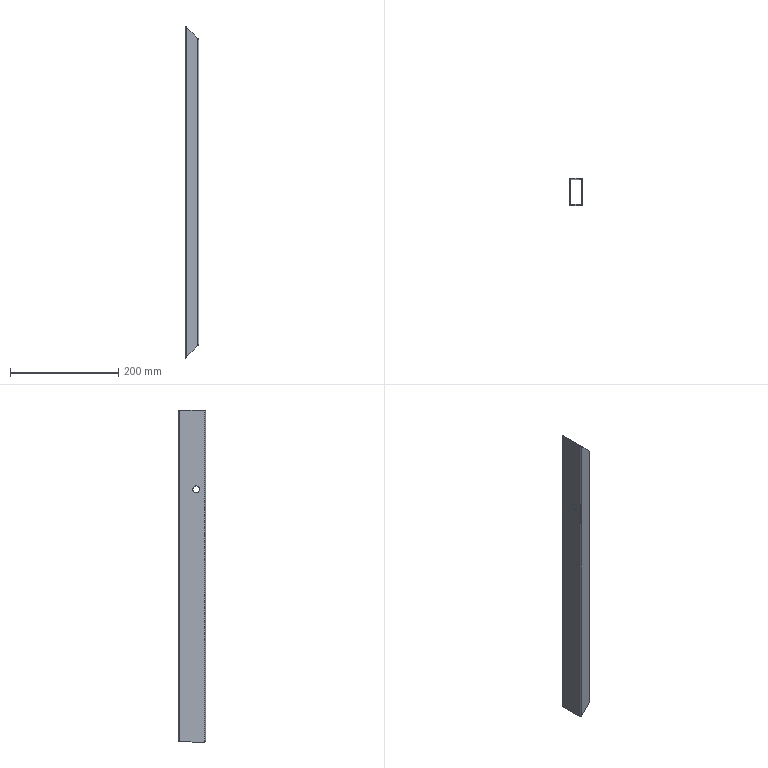Part | STEP file | 6150519 | 1 solid | 20 faces | box 25 x 50 x 613 mm | volume 123960 mm3 | cylinder 10 | plane 10 | commonest cylinder face diameters 2 x4 5 x4 13 x2
STEP:
#1=CARTESIAN_POINT('',(-10.,-25.,610.5));
#2=VERTEX_POINT('',#1);
#3=CARTESIAN_POINT('',(-10.,-25.,2.5));
#4=VERTEX_POINT('',#3);
#5=CARTESIAN_POINT('',(-10.,-25.,613.));
#6=DIRECTION('',(0.,0.,-1.));
#7=VECTOR('',#6,1000.);
#8=LINE('',#5,#7);
#9=EDGE_CURVE('',#2,#4,#8,.T.);
#10=ORIENTED_EDGE('',*,*,#9,.F.);
#11=CARTESIAN_POINT('',(-12.5,-22.5,613.));
#12=VERTEX_POINT('',#11);
#13=CARTESIAN_POINT('',(-10.,-25.,610.5));
#14=CARTESIAN_POINT('',(-11.464,-25.,611.964));
#15=CARTESIAN_POINT('',(-12.5,-23.964,613.));
#16=CARTESIAN_POINT('',(-12.5,-22.5,613.));
#17=(BOUNDED_CURVE()B_SPLINE_CURVE(3,(#13,#14,#15,#16),.UNSPECIFIED.,.F.,.F.)B_SPLINE_CURVE_WITH_KNOTS((4,4),(1.571,3.142),.UNSPECIFIED.)CURVE()GEOMETRIC_REPRESENTATION_ITEM()RATIONAL_B_SPLINE_CURVE((1.,0.8047,0.8047,1.))REPRESENTATION_ITEM(''));
#18=EDGE_CURVE('',#2,#12,#17,.T.);
#19=ORIENTED_EDGE('',*,*,#18,.T.);
#20=CARTESIAN_POINT('',(-12.5,-22.5,0.));
#21=VERTEX_POINT('',#20);
#22=CARTESIAN_POINT('',(-12.5,-22.5,613.));
#23=DIRECTION('',(0.,0.,-1.));
#24=VECTOR('',#23,1000.);
#25=LINE('',#22,#24);
#26=EDGE_CURVE('',#12,#21,#25,.T.);
#27=ORIENTED_EDGE('',*,*,#26,.T.);
#28=CARTESIAN_POINT('',(-10.,-25.,2.5));
#29=CARTESIAN_POINT('',(-11.464,-25.,1.036));
#30=CARTESIAN_POINT('',(-12.5,-23.964,0.));
#31=CARTESIAN_POINT('',(-12.5,-22.5,0.));
#32=(BOUNDED_CURVE()B_SPLINE_CURVE(3,(#28,#29,#30,#31),.UNSPECIFIED.,.F.,.F.)B_SPLINE_CURVE_WITH_KNOTS((4,4),(4.712,6.283),.UNSPECIFIED.)CURVE()GEOMETRIC_REPRESENTATION_ITEM()RATIONAL_B_SPLINE_CURVE((1.,0.8047,0.8047,1.))REPRESENTATION_ITEM(''));
#33=EDGE_CURVE('',#4,#21,#32,.T.);
#34=ORIENTED_EDGE('',*,*,#33,.F.);
#35=EDGE_LOOP('',(#10,#19,#27,#34));
#36=FACE_OUTER_BOUND('',#35,.T.);
#37=CARTESIAN_POINT('',(-10.,-22.5,613.));
#38=DIRECTION('',(0.,0.,-1.));
#39=DIRECTION('',(-1.,0.,0.));
#40=AXIS2_PLACEMENT_3D('',#37,#38,#39);
#41=CYLINDRICAL_SURFACE('',#40,2.5);
#42=ADVANCED_FACE('',(#36),#41,.T.);
#43=CARTESIAN_POINT('',(10.,-25.,590.5));
#44=VERTEX_POINT('',#43);
#45=CARTESIAN_POINT('',(10.,-25.,22.5));
#46=VERTEX_POINT('',#45);
#47=CARTESIAN_POINT('',(10.,-25.,613.));
#48=DIRECTION('',(0.,0.,-1.));
#49=VECTOR('',#48,1000.);
#50=LINE('',#47,#49);
#51=EDGE_CURVE('',#44,#46,#50,.T.);
#52=ORIENTED_EDGE('',*,*,#51,.F.);
#53=CARTESIAN_POINT('',(-11.25,-25.,611.75));
#54=DIRECTION('',(-0.7071,0.,0.7071));
#55=VECTOR('',#54,1000.);
#56=LINE('',#53,#55);
#57=EDGE_CURVE('',#44,#2,#56,.T.);
#58=ORIENTED_EDGE('',*,*,#57,.T.);
#59=ORIENTED_EDGE('',*,*,#9,.T.);
#60=CARTESIAN_POINT('',(295.25,-25.,307.75));
#61=DIRECTION('',(-0.7071,0.,-0.7071));
#62=VECTOR('',#61,1000.);
#63=LINE('',#60,#62);
#64=EDGE_CURVE('',#46,#4,#63,.T.);
#65=ORIENTED_EDGE('',*,*,#64,.F.);
#66=EDGE_LOOP('',(#52,#58,#59,#65));
#67=FACE_OUTER_BOUND('',#66,.T.);
#68=CARTESIAN_POINT('',(-10.,-25.,613.));
#69=DIRECTION('',(0.,1.,0.));
#70=DIRECTION('',(0.,0.,1.));
#71=AXIS2_PLACEMENT_3D('',#68,#69,#70);
#72=PLANE('',#71);
#73=ADVANCED_FACE('',(#67),#72,.F.);
#74=CARTESIAN_POINT('',(12.5,-22.5,588.));
#75=VERTEX_POINT('',#74);
#76=CARTESIAN_POINT('',(12.5,-22.5,25.));
#77=VERTEX_POINT('',#76);
#78=CARTESIAN_POINT('',(12.5,-22.5,613.));
#79=DIRECTION('',(0.,0.,-1.));
#80=VECTOR('',#79,1000.);
#81=LINE('',#78,#80);
#82=EDGE_CURVE('',#75,#77,#81,.T.);
#83=ORIENTED_EDGE('',*,*,#82,.F.);
#84=CARTESIAN_POINT('',(12.5,-22.5,588.));
#85=CARTESIAN_POINT('',(12.5,-23.964,588.));
#86=CARTESIAN_POINT('',(11.464,-25.,589.036));
#87=CARTESIAN_POINT('',(10.,-25.,590.5));
#88=(BOUNDED_CURVE()B_SPLINE_CURVE(3,(#84,#85,#86,#87),.UNSPECIFIED.,.F.,.T.)B_SPLINE_CURVE_WITH_KNOTS((4,4),(0.,1.571),.UNSPECIFIED.)CURVE()GEOMETRIC_REPRESENTATION_ITEM()RATIONAL_B_SPLINE_CURVE((1.,0.8047,0.8047,1.))REPRESENTATION_ITEM(''));
#89=EDGE_CURVE('',#75,#44,#88,.T.);
#90=ORIENTED_EDGE('',*,*,#89,.T.);
#91=ORIENTED_EDGE('',*,*,#51,.T.);
#92=CARTESIAN_POINT('',(12.5,-22.5,25.));
#93=CARTESIAN_POINT('',(12.5,-23.964,25.));
#94=CARTESIAN_POINT('',(11.464,-25.,23.964));
#95=CARTESIAN_POINT('',(10.,-25.,22.5));
#96=(BOUNDED_CURVE()B_SPLINE_CURVE(3,(#92,#93,#94,#95),.UNSPECIFIED.,.F.,.F.)B_SPLINE_CURVE_WITH_KNOTS((4,4),(3.142,4.712),.UNSPECIFIED.)CURVE()GEOMETRIC_REPRESENTATION_ITEM()RATIONAL_B_SPLINE_CURVE((1.,0.8047,0.8047,1.))REPRESENTATION_ITEM(''));
#97=EDGE_CURVE('',#77,#46,#96,.T.);
#98=ORIENTED_EDGE('',*,*,#97,.F.);
#99=EDGE_LOOP('',(#83,#90,#91,#98));
#100=FACE_OUTER_BOUND('',#99,.T.);
#101=CARTESIAN_POINT('',(10.,-22.5,613.));
#102=DIRECTION('',(0.,0.,-1.));
#103=DIRECTION('',(-1.,0.,0.));
#104=AXIS2_PLACEMENT_3D('',#101,#102,#103);
#105=CYLINDRICAL_SURFACE('',#104,2.5);
#106=ADVANCED_FACE('',(#100),#105,.T.);
#107=CARTESIAN_POINT('',(12.5,-14.5,466.5));
#108=VERTEX_POINT('',#107);
#109=CARTESIAN_POINT('',(12.5,-8.,466.5));
#110=DIRECTION('',(-1.,0.,0.));
#111=DIRECTION('',(0.,-1.,0.));
#112=AXIS2_PLACEMENT_3D('',#109,#110,#111);
#113=CIRCLE('',#112,6.5);
#114=EDGE_CURVE('',#108,#108,#113,.T.);
#115=ORIENTED_EDGE('',*,*,#114,.T.);
#116=EDGE_LOOP('',(#115));
#117=FACE_BOUND('',#116,.T.);
#118=CARTESIAN_POINT('',(12.5,22.5,588.));
#119=VERTEX_POINT('',#118);
#120=CARTESIAN_POINT('',(12.5,22.5,25.));
#121=VERTEX_POINT('',#120);
#122=CARTESIAN_POINT('',(12.5,22.5,613.));
#123=DIRECTION('',(0.,0.,-1.));
#124=VECTOR('',#123,1000.);
#125=LINE('',#122,#124);
#126=EDGE_CURVE('',#119,#121,#125,.T.);
#127=ORIENTED_EDGE('',*,*,#126,.F.);
#128=CARTESIAN_POINT('',(12.5,22.5,588.));
#129=DIRECTION('',(0.,-1.,0.));
#130=VECTOR('',#129,1000.);
#131=LINE('',#128,#130);
#132=EDGE_CURVE('',#119,#75,#131,.T.);
#133=ORIENTED_EDGE('',*,*,#132,.T.);
#134=ORIENTED_EDGE('',*,*,#82,.T.);
#135=CARTESIAN_POINT('',(12.5,22.5,25.));
#136=DIRECTION('',(0.,-1.,0.));
#137=VECTOR('',#136,1000.);
#138=LINE('',#135,#137);
#139=EDGE_CURVE('',#121,#77,#138,.T.);
#140=ORIENTED_EDGE('',*,*,#139,.F.);
#141=EDGE_LOOP('',(#127,#133,#134,#140));
#142=FACE_OUTER_BOUND('',#141,.T.);
#143=CARTESIAN_POINT('',(12.5,22.5,613.));
#144=DIRECTION('',(-1.,0.,0.));
#145=DIRECTION('',(0.,-1.,0.));
#146=AXIS2_PLACEMENT_3D('',#143,#144,#145);
#147=PLANE('',#146);
#148=ADVANCED_FACE('',(#117,#142),#147,.F.);
#149=CARTESIAN_POINT('',(10.,25.,590.5));
#150=VERTEX_POINT('',#149);
#151=CARTESIAN_POINT('',(10.,25.,22.5));
#152=VERTEX_POINT('',#151);
#153=CARTESIAN_POINT('',(10.,25.,613.));
#154=DIRECTION('',(0.,0.,-1.));
#155=VECTOR('',#154,1000.);
#156=LINE('',#153,#155);
#157=EDGE_CURVE('',#150,#152,#156,.T.);
#158=ORIENTED_EDGE('',*,*,#157,.F.);
#159=CARTESIAN_POINT('',(10.,25.,590.5));
#160=CARTESIAN_POINT('',(11.464,25.,589.036));
#161=CARTESIAN_POINT('',(12.5,23.964,588.));
#162=CARTESIAN_POINT('',(12.5,22.5,588.));
#163=(BOUNDED_CURVE()B_SPLINE_CURVE(3,(#159,#160,#161,#162),.UNSPECIFIED.,.F.,.F.)B_SPLINE_CURVE_WITH_KNOTS((4,4),(4.712,6.283),.UNSPECIFIED.)CURVE()GEOMETRIC_REPRESENTATION_ITEM()RATIONAL_B_SPLINE_CURVE((1.,0.8047,0.8047,1.))REPRESENTATION_ITEM(''));
#164=EDGE_CURVE('',#150,#119,#163,.T.);
#165=ORIENTED_EDGE('',*,*,#164,.T.);
#166=ORIENTED_EDGE('',*,*,#126,.T.);
#167=CARTESIAN_POINT('',(10.,25.,22.5));
#168=CARTESIAN_POINT('',(11.464,25.,23.964));
#169=CARTESIAN_POINT('',(12.5,23.964,25.));
#170=CARTESIAN_POINT('',(12.5,22.5,25.));
#171=(BOUNDED_CURVE()B_SPLINE_CURVE(3,(#167,#168,#169,#170),.UNSPECIFIED.,.F.,.F.)B_SPLINE_CURVE_WITH_KNOTS((4,4),(1.571,3.142),.UNSPECIFIED.)CURVE()GEOMETRIC_REPRESENTATION_ITEM()RATIONAL_B_SPLINE_CURVE((1.,0.8047,0.8047,1.))REPRESENTATION_ITEM(''));
#172=EDGE_CURVE('',#152,#121,#171,.T.);
#173=ORIENTED_EDGE('',*,*,#172,.F.);
#174=EDGE_LOOP('',(#158,#165,#166,#173));
#175=FACE_OUTER_BOUND('',#174,.T.);
#176=CARTESIAN_POINT('',(10.,22.5,613.));
#177=DIRECTION('',(0.,0.,-1.));
#178=DIRECTION('',(-1.,0.,0.));
#179=AXIS2_PLACEMENT_3D('',#176,#177,#178);
#180=CYLINDRICAL_SURFACE('',#179,2.5);
#181=ADVANCED_FACE('',(#175),#180,.T.);
#182=CARTESIAN_POINT('',(-10.,25.,610.5));
#183=VERTEX_POINT('',#182);
#184=CARTESIAN_POINT('',(-10.,25.,2.5));
#185=VERTEX_POINT('',#184);
#186=CARTESIAN_POINT('',(-10.,25.,613.));
#187=DIRECTION('',(0.,0.,-1.));
#188=VECTOR('',#187,1000.);
#189=LINE('',#186,#188);
#190=EDGE_CURVE('',#183,#185,#189,.T.);
#191=ORIENTED_EDGE('',*,*,#190,.F.);
#192=CARTESIAN_POINT('',(-11.25,25.,611.75));
#193=DIRECTION('',(0.7071,0.,-0.7071));
#194=VECTOR('',#193,1000.);
#195=LINE('',#192,#194);
#196=EDGE_CURVE('',#183,#150,#195,.T.);
#197=ORIENTED_EDGE('',*,*,#196,.T.);
#198=ORIENTED_EDGE('',*,*,#157,.T.);
#199=CARTESIAN_POINT('',(295.25,25.,307.75));
#200=DIRECTION('',(0.7071,0.,0.7071));
#201=VECTOR('',#200,1000.);
#202=LINE('',#199,#201);
#203=EDGE_CURVE('',#185,#152,#202,.T.);
#204=ORIENTED_EDGE('',*,*,#203,.F.);
#205=EDGE_LOOP('',(#191,#197,#198,#204));
#206=FACE_OUTER_BOUND('',#205,.T.);
#207=CARTESIAN_POINT('',(-10.,25.,613.));
#208=DIRECTION('',(0.,-1.,0.));
#209=DIRECTION('',(0.,0.,-1.));
#210=AXIS2_PLACEMENT_3D('',#207,#208,#209);
#211=PLANE('',#210);
#212=ADVANCED_FACE('',(#206),#211,.F.);
#213=CARTESIAN_POINT('',(-12.5,22.5,613.));
#214=VERTEX_POINT('',#213);
#215=CARTESIAN_POINT('',(-12.5,22.5,0.));
#216=VERTEX_POINT('',#215);
#217=CARTESIAN_POINT('',(-12.5,22.5,613.));
#218=DIRECTION('',(0.,0.,-1.));
#219=VECTOR('',#218,1000.);
#220=LINE('',#217,#219);
#221=EDGE_CURVE('',#214,#216,#220,.T.);
#222=ORIENTED_EDGE('',*,*,#221,.F.);
#223=CARTESIAN_POINT('',(-12.5,22.5,613.));
#224=CARTESIAN_POINT('',(-12.5,23.964,613.));
#225=CARTESIAN_POINT('',(-11.464,25.,611.964));
#226=CARTESIAN_POINT('',(-10.,25.,610.5));
#227=(BOUNDED_CURVE()B_SPLINE_CURVE(3,(#223,#224,#225,#226),.UNSPECIFIED.,.F.,.F.)B_SPLINE_CURVE_WITH_KNOTS((4,4),(3.142,4.712),.UNSPECIFIED.)CURVE()GEOMETRIC_REPRESENTATION_ITEM()RATIONAL_B_SPLINE_CURVE((1.,0.8047,0.8047,1.))REPRESENTATION_ITEM(''));
#228=EDGE_CURVE('',#214,#183,#227,.T.);
#229=ORIENTED_EDGE('',*,*,#228,.T.);
#230=ORIENTED_EDGE('',*,*,#190,.T.);
#231=CARTESIAN_POINT('',(-12.5,22.5,0.));
#232=CARTESIAN_POINT('',(-12.5,23.964,0.));
#233=CARTESIAN_POINT('',(-11.464,25.,1.036));
#234=CARTESIAN_POINT('',(-10.,25.,2.5));
#235=(BOUNDED_CURVE()B_SPLINE_CURVE(3,(#231,#232,#233,#234),.UNSPECIFIED.,.F.,.F.)B_SPLINE_CURVE_WITH_KNOTS((4,4),(0.,1.571),.UNSPECIFIED.)CURVE()GEOMETRIC_REPRESENTATION_ITEM()RATIONAL_B_SPLINE_CURVE((1.,0.8047,0.8047,1.))REPRESENTATION_ITEM(''));
#236=EDGE_CURVE('',#216,#185,#235,.T.);
#237=ORIENTED_EDGE('',*,*,#236,.F.);
#238=EDGE_LOOP('',(#222,#229,#230,#237));
#239=FACE_OUTER_BOUND('',#238,.T.);
#240=CARTESIAN_POINT('',(-10.,22.5,613.));
#241=DIRECTION('',(0.,0.,-1.));
#242=DIRECTION('',(-1.,0.,0.));
#243=AXIS2_PLACEMENT_3D('',#240,#241,#242);
#244=CYLINDRICAL_SURFACE('',#243,2.5);
#245=ADVANCED_FACE('',(#239),#244,.T.);
#246=CARTESIAN_POINT('',(10.,23.5,590.5));
#247=VERTEX_POINT('',#246);
#248=CARTESIAN_POINT('',(11.,22.5,589.5));
#249=VERTEX_POINT('',#248);
#250=CARTESIAN_POINT('',(10.,23.5,590.5));
#251=CARTESIAN_POINT('',(10.586,23.5,589.914));
#252=CARTESIAN_POINT('',(11.,23.086,589.5));
#253=CARTESIAN_POINT('',(11.,22.5,589.5));
#254=(BOUNDED_CURVE()B_SPLINE_CURVE(3,(#250,#251,#252,#253),.UNSPECIFIED.,.F.,.F.)B_SPLINE_CURVE_WITH_KNOTS((4,4),(4.712,6.283),.UNSPECIFIED.)CURVE()GEOMETRIC_REPRESENTATION_ITEM()RATIONAL_B_SPLINE_CURVE((1.,0.8047,0.8047,1.))REPRESENTATION_ITEM(''));
#255=EDGE_CURVE('',#247,#249,#254,.T.);
#256=ORIENTED_EDGE('',*,*,#255,.F.);
#257=CARTESIAN_POINT('',(10.,23.5,22.5));
#258=VERTEX_POINT('',#257);
#259=CARTESIAN_POINT('',(10.,23.5,613.));
#260=DIRECTION('',(0.,0.,-1.));
#261=VECTOR('',#260,1000.);
#262=LINE('',#259,#261);
#263=EDGE_CURVE('',#247,#258,#262,.T.);
#264=ORIENTED_EDGE('',*,*,#263,.T.);
#265=CARTESIAN_POINT('',(11.,22.5,23.5));
#266=VERTEX_POINT('',#265);
#267=CARTESIAN_POINT('',(10.,23.5,22.5));
#268=CARTESIAN_POINT('',(10.586,23.5,23.086));
#269=CARTESIAN_POINT('',(11.,23.086,23.5));
#270=CARTESIAN_POINT('',(11.,22.5,23.5));
#271=(BOUNDED_CURVE()B_SPLINE_CURVE(3,(#267,#268,#269,#270),.UNSPECIFIED.,.F.,.F.)B_SPLINE_CURVE_WITH_KNOTS((4,4),(1.571,3.142),.UNSPECIFIED.)CURVE()GEOMETRIC_REPRESENTATION_ITEM()RATIONAL_B_SPLINE_CURVE((1.,0.8047,0.8047,1.))REPRESENTATION_ITEM(''));
#272=EDGE_CURVE('',#258,#266,#271,.T.);
#273=ORIENTED_EDGE('',*,*,#272,.T.);
#274=CARTESIAN_POINT('',(11.,22.5,613.));
#275=DIRECTION('',(0.,0.,-1.));
#276=VECTOR('',#275,1000.);
#277=LINE('',#274,#276);
#278=EDGE_CURVE('',#249,#266,#277,.T.);
#279=ORIENTED_EDGE('',*,*,#278,.F.);
#280=EDGE_LOOP('',(#256,#264,#273,#279));
#281=FACE_OUTER_BOUND('',#280,.T.);
#282=CARTESIAN_POINT('',(10.,22.5,613.));
#283=DIRECTION('',(0.,0.,-1.));
#284=DIRECTION('',(-1.,0.,0.));
#285=AXIS2_PLACEMENT_3D('',#282,#283,#284);
#286=CYLINDRICAL_SURFACE('',#285,1.);
#287=ADVANCED_FACE('',(#281),#286,.F.);
#288=CARTESIAN_POINT('',(-10.,23.5,610.5));
#289=VERTEX_POINT('',#288);
#290=CARTESIAN_POINT('',(-11.25,23.5,611.75));
#291=DIRECTION('',(0.7071,0.,-0.7071));
#292=VECTOR('',#291,1000.);
#293=LINE('',#290,#292);
#294=EDGE_CURVE('',#289,#247,#293,.T.);
#295=ORIENTED_EDGE('',*,*,#294,.F.);
#296=CARTESIAN_POINT('',(-10.,23.5,2.5));
#297=VERTEX_POINT('',#296);
#298=CARTESIAN_POINT('',(-10.,23.5,613.));
#299=DIRECTION('',(0.,0.,-1.));
#300=VECTOR('',#299,1000.);
#301=LINE('',#298,#300);
#302=EDGE_CURVE('',#289,#297,#301,.T.);
#303=ORIENTED_EDGE('',*,*,#302,.T.);
#304=CARTESIAN_POINT('',(295.25,23.5,307.75));
#305=DIRECTION('',(0.7071,0.,0.7071));
#306=VECTOR('',#305,1000.);
#307=LINE('',#304,#306);
#308=EDGE_CURVE('',#297,#258,#307,.T.);
#309=ORIENTED_EDGE('',*,*,#308,.T.);
#310=ORIENTED_EDGE('',*,*,#263,.F.);
#311=EDGE_LOOP('',(#295,#303,#309,#310));
#312=FACE_OUTER_BOUND('',#311,.T.);
#313=CARTESIAN_POINT('',(-10.,23.5,613.));
#314=DIRECTION('',(0.,-1.,0.));
#315=DIRECTION('',(1.,0.,0.));
#316=AXIS2_PLACEMENT_3D('',#313,#314,#315);
#317=PLANE('',#316);
#318=ADVANCED_FACE('',(#312),#317,.T.);
#319=CARTESIAN_POINT('',(-11.,22.5,611.5));
#320=VERTEX_POINT('',#319);
#321=CARTESIAN_POINT('',(-11.,22.5,611.5));
#322=CARTESIAN_POINT('',(-11.,23.086,611.5));
#323=CARTESIAN_POINT('',(-10.586,23.5,611.086));
#324=CARTESIAN_POINT('',(-10.,23.5,610.5));
#325=(BOUNDED_CURVE()B_SPLINE_CURVE(3,(#321,#322,#323,#324),.UNSPECIFIED.,.F.,.F.)B_SPLINE_CURVE_WITH_KNOTS((4,4),(3.142,4.712),.UNSPECIFIED.)CURVE()GEOMETRIC_REPRESENTATION_ITEM()RATIONAL_B_SPLINE_CURVE((1.,0.8047,0.8047,1.))REPRESENTATION_ITEM(''));
#326=EDGE_CURVE('',#320,#289,#325,.T.);
#327=ORIENTED_EDGE('',*,*,#326,.F.);
#328=CARTESIAN_POINT('',(-11.,22.5,1.5));
#329=VERTEX_POINT('',#328);
#330=CARTESIAN_POINT('',(-11.,22.5,613.));
#331=DIRECTION('',(0.,0.,-1.));
#332=VECTOR('',#331,1000.);
#333=LINE('',#330,#332);
#334=EDGE_CURVE('',#320,#329,#333,.T.);
#335=ORIENTED_EDGE('',*,*,#334,.T.);
#336=CARTESIAN_POINT('',(-11.,22.5,1.5));
#337=CARTESIAN_POINT('',(-11.,23.086,1.5));
#338=CARTESIAN_POINT('',(-10.586,23.5,1.914));
#339=CARTESIAN_POINT('',(-10.,23.5,2.5));
#340=(BOUNDED_CURVE()B_SPLINE_CURVE(3,(#336,#337,#338,#339),.UNSPECIFIED.,.F.,.F.)B_SPLINE_CURVE_WITH_KNOTS((4,4),(0.,1.571),.UNSPECIFIED.)CURVE()GEOMETRIC_REPRESENTATION_ITEM()RATIONAL_B_SPLINE_CURVE((1.,0.8047,0.8047,1.))REPRESENTATION_ITEM(''));
#341=EDGE_CURVE('',#329,#297,#340,.T.);
#342=ORIENTED_EDGE('',*,*,#341,.T.);
#343=ORIENTED_EDGE('',*,*,#302,.F.);
#344=EDGE_LOOP('',(#327,#335,#342,#343));
#345=FACE_OUTER_BOUND('',#344,.T.);
#346=CARTESIAN_POINT('',(-10.,22.5,613.));
#347=DIRECTION('',(0.,0.,-1.));
#348=DIRECTION('',(-1.,0.,0.));
#349=AXIS2_PLACEMENT_3D('',#346,#347,#348);
#350=CYLINDRICAL_SURFACE('',#349,1.);
#351=ADVANCED_FACE('',(#345),#350,.F.);
#352=CARTESIAN_POINT('',(-11.,-1.5,466.5));
#353=VERTEX_POINT('',#352);
#354=CARTESIAN_POINT('',(-11.,-8.,466.5));
#355=DIRECTION('',(1.,0.,0.));
#356=DIRECTION('',(0.,1.,0.));
#357=AXIS2_PLACEMENT_3D('',#354,#355,#356);
#358=CIRCLE('',#357,6.5);
#359=EDGE_CURVE('',#353,#353,#358,.T.);
#360=ORIENTED_EDGE('',*,*,#359,.F.);
#361=EDGE_LOOP('',(#360));
#362=FACE_BOUND('',#361,.T.);
#363=CARTESIAN_POINT('',(-11.,-22.5,611.5));
#364=VERTEX_POINT('',#363);
#365=CARTESIAN_POINT('',(-11.,22.5,611.5));
#366=DIRECTION('',(0.,1.,0.));
#367=VECTOR('',#366,1000.);
#368=LINE('',#365,#367);
#369=EDGE_CURVE('',#364,#320,#368,.T.);
#370=ORIENTED_EDGE('',*,*,#369,.F.);
#371=CARTESIAN_POINT('',(-11.,-22.5,1.5));
#372=VERTEX_POINT('',#371);
#373=CARTESIAN_POINT('',(-11.,-22.5,613.));
#374=DIRECTION('',(0.,0.,-1.));
#375=VECTOR('',#374,1000.);
#376=LINE('',#373,#375);
#377=EDGE_CURVE('',#364,#372,#376,.T.);
#378=ORIENTED_EDGE('',*,*,#377,.T.);
#379=CARTESIAN_POINT('',(-11.,22.5,1.5));
#380=DIRECTION('',(0.,1.,0.));
#381=VECTOR('',#380,1000.);
#382=LINE('',#379,#381);
#383=EDGE_CURVE('',#372,#329,#382,.T.);
#384=ORIENTED_EDGE('',*,*,#383,.T.);
#385=ORIENTED_EDGE('',*,*,#334,.F.);
#386=EDGE_LOOP('',(#370,#378,#384,#385));
#387=FACE_OUTER_BOUND('',#386,.T.);
#388=CARTESIAN_POINT('',(-11.,22.5,613.));
#389=DIRECTION('',(1.,0.,0.));
#390=DIRECTION('',(0.,1.,0.));
#391=AXIS2_PLACEMENT_3D('',#388,#389,#390);
#392=PLANE('',#391);
#393=ADVANCED_FACE('',(#362,#387),#392,.T.);
#394=CARTESIAN_POINT('',(-10.,-23.5,610.5));
#395=VERTEX_POINT('',#394);
#396=CARTESIAN_POINT('',(-10.,-23.5,610.5));
#397=CARTESIAN_POINT('',(-10.586,-23.5,611.086));
#398=CARTESIAN_POINT('',(-11.,-23.086,611.5));
#399=CARTESIAN_POINT('',(-11.,-22.5,611.5));
#400=(BOUNDED_CURVE()B_SPLINE_CURVE(3,(#396,#397,#398,#399),.UNSPECIFIED.,.F.,.T.)B_SPLINE_CURVE_WITH_KNOTS((4,4),(1.571,3.142),.UNSPECIFIED.)CURVE()GEOMETRIC_REPRESENTATION_ITEM()RATIONAL_B_SPLINE_CURVE((1.,0.8047,0.8047,1.))REPRESENTATION_ITEM(''));
#401=EDGE_CURVE('',#395,#364,#400,.T.);
#402=ORIENTED_EDGE('',*,*,#401,.F.);
#403=CARTESIAN_POINT('',(-10.,-23.5,2.5));
#404=VERTEX_POINT('',#403);
#405=CARTESIAN_POINT('',(-10.,-23.5,613.));
#406=DIRECTION('',(0.,0.,-1.));
#407=VECTOR('',#406,1000.);
#408=LINE('',#405,#407);
#409=EDGE_CURVE('',#395,#404,#408,.T.);
#410=ORIENTED_EDGE('',*,*,#409,.T.);
#411=CARTESIAN_POINT('',(-10.,-23.5,2.5));
#412=CARTESIAN_POINT('',(-10.586,-23.5,1.914));
#413=CARTESIAN_POINT('',(-11.,-23.086,1.5));
#414=CARTESIAN_POINT('',(-11.,-22.5,1.5));
#415=(BOUNDED_CURVE()B_SPLINE_CURVE(3,(#411,#412,#413,#414),.UNSPECIFIED.,.F.,.F.)B_SPLINE_CURVE_WITH_KNOTS((4,4),(4.712,6.283),.UNSPECIFIED.)CURVE()GEOMETRIC_REPRESENTATION_ITEM()RATIONAL_B_SPLINE_CURVE((1.,0.8047,0.8047,1.))REPRESENTATION_ITEM(''));
#416=EDGE_CURVE('',#404,#372,#415,.T.);
#417=ORIENTED_EDGE('',*,*,#416,.T.);
#418=ORIENTED_EDGE('',*,*,#377,.F.);
#419=EDGE_LOOP('',(#402,#410,#417,#418));
#420=FACE_OUTER_BOUND('',#419,.T.);
#421=CARTESIAN_POINT('',(-10.,-22.5,613.));
#422=DIRECTION('',(0.,0.,-1.));
#423=DIRECTION('',(-1.,0.,0.));
#424=AXIS2_PLACEMENT_3D('',#421,#422,#423);
#425=CYLINDRICAL_SURFACE('',#424,1.);
#426=ADVANCED_FACE('',(#420),#425,.F.);
#427=CARTESIAN_POINT('',(10.,-23.5,590.5));
#428=VERTEX_POINT('',#427);
#429=CARTESIAN_POINT('',(-11.25,-23.5,611.75));
#430=DIRECTION('',(-0.7071,0.,0.7071));
#431=VECTOR('',#430,1000.);
#432=LINE('',#429,#431);
#433=EDGE_CURVE('',#428,#395,#432,.T.);
#434=ORIENTED_EDGE('',*,*,#433,.F.);
#435=CARTESIAN_POINT('',(10.,-23.5,22.5));
#436=VERTEX_POINT('',#435);
#437=CARTESIAN_POINT('',(10.,-23.5,613.));
#438=DIRECTION('',(0.,0.,-1.));
#439=VECTOR('',#438,1000.);
#440=LINE('',#437,#439);
#441=EDGE_CURVE('',#428,#436,#440,.T.);
#442=ORIENTED_EDGE('',*,*,#441,.T.);
#443=CARTESIAN_POINT('',(295.25,-23.5,307.75));
#444=DIRECTION('',(-0.7071,0.,-0.7071));
#445=VECTOR('',#444,1000.);
#446=LINE('',#443,#445);
#447=EDGE_CURVE('',#436,#404,#446,.T.);
#448=ORIENTED_EDGE('',*,*,#447,.T.);
#449=ORIENTED_EDGE('',*,*,#409,.F.);
#450=EDGE_LOOP('',(#434,#442,#448,#449));
#451=FACE_OUTER_BOUND('',#450,.T.);
#452=CARTESIAN_POINT('',(-10.,-23.5,613.));
#453=DIRECTION('',(0.,1.,0.));
#454=DIRECTION('',(-1.,0.,0.));
#455=AXIS2_PLACEMENT_3D('',#452,#453,#454);
#456=PLANE('',#455);
#457=ADVANCED_FACE('',(#451),#456,.T.);
#458=CARTESIAN_POINT('',(11.,-22.5,589.5));
#459=VERTEX_POINT('',#458);
#460=CARTESIAN_POINT('',(11.,-22.5,589.5));
#461=CARTESIAN_POINT('',(11.,-23.086,589.5));
#462=CARTESIAN_POINT('',(10.586,-23.5,589.914));
#463=CARTESIAN_POINT('',(10.,-23.5,590.5));
#464=(BOUNDED_CURVE()B_SPLINE_CURVE(3,(#460,#461,#462,#463),.UNSPECIFIED.,.F.,.T.)B_SPLINE_CURVE_WITH_KNOTS((4,4),(0.,1.571),.UNSPECIFIED.)CURVE()GEOMETRIC_REPRESENTATION_ITEM()RATIONAL_B_SPLINE_CURVE((1.,0.8047,0.8047,1.))REPRESENTATION_ITEM(''));
#465=EDGE_CURVE('',#459,#428,#464,.T.);
#466=ORIENTED_EDGE('',*,*,#465,.F.);
#467=CARTESIAN_POINT('',(11.,-22.5,23.5));
#468=VERTEX_POINT('',#467);
#469=CARTESIAN_POINT('',(11.,-22.5,613.));
#470=DIRECTION('',(0.,0.,-1.));
#471=VECTOR('',#470,1000.);
#472=LINE('',#469,#471);
#473=EDGE_CURVE('',#459,#468,#472,.T.);
#474=ORIENTED_EDGE('',*,*,#473,.T.);
#475=CARTESIAN_POINT('',(11.,-22.5,23.5));
#476=CARTESIAN_POINT('',(11.,-23.086,23.5));
#477=CARTESIAN_POINT('',(10.586,-23.5,23.086));
#478=CARTESIAN_POINT('',(10.,-23.5,22.5));
#479=(BOUNDED_CURVE()B_SPLINE_CURVE(3,(#475,#476,#477,#478),.UNSPECIFIED.,.F.,.F.)B_SPLINE_CURVE_WITH_KNOTS((4,4),(3.142,4.712),.UNSPECIFIED.)CURVE()GEOMETRIC_REPRESENTATION_ITEM()RATIONAL_B_SPLINE_CURVE((1.,0.8047,0.8047,1.))REPRESENTATION_ITEM(''));
#480=EDGE_CURVE('',#468,#436,#479,.T.);
#481=ORIENTED_EDGE('',*,*,#480,.T.);
#482=ORIENTED_EDGE('',*,*,#441,.F.);
#483=EDGE_LOOP('',(#466,#474,#481,#482));
#484=FACE_OUTER_BOUND('',#483,.T.);
#485=CARTESIAN_POINT('',(10.,-22.5,613.));
#486=DIRECTION('',(0.,0.,-1.));
#487=DIRECTION('',(-1.,0.,0.));
#488=AXIS2_PLACEMENT_3D('',#485,#486,#487);
#489=CYLINDRICAL_SURFACE('',#488,1.);
#490=ADVANCED_FACE('',(#484),#489,.F.);
#491=CARTESIAN_POINT('',(11.,-8.,473.));
#492=VERTEX_POINT('',#491);
#493=CARTESIAN_POINT('',(11.,-8.,466.5));
#494=DIRECTION('',(-1.,0.,0.));
#495=DIRECTION('',(0.,0.,1.));
#496=AXIS2_PLACEMENT_3D('',#493,#494,#495);
#497=CIRCLE('',#496,6.5);
#498=EDGE_CURVE('',#492,#492,#497,.T.);
#499=ORIENTED_EDGE('',*,*,#498,.F.);
#500=EDGE_LOOP('',(#499));
#501=FACE_BOUND('',#500,.T.);
#502=CARTESIAN_POINT('',(11.,22.5,589.5));
#503=DIRECTION('',(0.,-1.,0.));
#504=VECTOR('',#503,1000.);
#505=LINE('',#502,#504);
#506=EDGE_CURVE('',#249,#459,#505,.T.);
#507=ORIENTED_EDGE('',*,*,#506,.F.);
#508=ORIENTED_EDGE('',*,*,#278,.T.);
#509=CARTESIAN_POINT('',(11.,22.5,23.5));
#510=DIRECTION('',(0.,-1.,0.));
#511=VECTOR('',#510,1000.);
#512=LINE('',#509,#511);
#513=EDGE_CURVE('',#266,#468,#512,.T.);
#514=ORIENTED_EDGE('',*,*,#513,.T.);
#515=ORIENTED_EDGE('',*,*,#473,.F.);
#516=EDGE_LOOP('',(#507,#508,#514,#515));
#517=FACE_OUTER_BOUND('',#516,.T.);
#518=CARTESIAN_POINT('',(11.,22.5,613.));
#519=DIRECTION('',(-1.,0.,0.));
#520=DIRECTION('',(0.,0.,1.));
#521=AXIS2_PLACEMENT_3D('',#518,#519,#520);
#522=PLANE('',#521);
#523=ADVANCED_FACE('',(#501,#517),#522,.T.);
#524=CARTESIAN_POINT('',(-12.5,-14.5,466.5));
#525=VERTEX_POINT('',#524);
#526=CARTESIAN_POINT('',(-12.5,-8.,466.5));
#527=DIRECTION('',(-1.,0.,0.));
#528=DIRECTION('',(0.,-1.,0.));
#529=AXIS2_PLACEMENT_3D('',#526,#527,#528);
#530=CIRCLE('',#529,6.5);
#531=EDGE_CURVE('',#525,#525,#530,.T.);
#532=ORIENTED_EDGE('',*,*,#531,.F.);
#533=EDGE_LOOP('',(#532));
#534=FACE_BOUND('',#533,.T.);
#535=CARTESIAN_POINT('',(-12.5,22.5,0.));
#536=DIRECTION('',(0.,-1.,0.));
#537=VECTOR('',#536,1000.);
#538=LINE('',#535,#537);
#539=EDGE_CURVE('',#216,#21,#538,.T.);
#540=ORIENTED_EDGE('',*,*,#539,.T.);
#541=ORIENTED_EDGE('',*,*,#26,.F.);
#542=CARTESIAN_POINT('',(-12.5,22.5,613.));
#543=DIRECTION('',(0.,-1.,0.));
#544=VECTOR('',#543,1000.);
#545=LINE('',#542,#544);
#546=EDGE_CURVE('',#214,#12,#545,.T.);
#547=ORIENTED_EDGE('',*,*,#546,.F.);
#548=ORIENTED_EDGE('',*,*,#221,.T.);
#549=EDGE_LOOP('',(#540,#541,#547,#548));
#550=FACE_OUTER_BOUND('',#549,.T.);
#551=CARTESIAN_POINT('',(-12.5,22.5,613.));
#552=DIRECTION('',(1.,0.,0.));
#553=DIRECTION('',(0.,1.,0.));
#554=AXIS2_PLACEMENT_3D('',#551,#552,#553);
#555=PLANE('',#554);
#556=ADVANCED_FACE('',(#534,#550),#555,.F.);
#557=ORIENTED_EDGE('',*,*,#272,.F.);
#558=ORIENTED_EDGE('',*,*,#308,.F.);
#559=ORIENTED_EDGE('',*,*,#341,.F.);
#560=ORIENTED_EDGE('',*,*,#383,.F.);
#561=ORIENTED_EDGE('',*,*,#416,.F.);
#562=ORIENTED_EDGE('',*,*,#447,.F.);
#563=ORIENTED_EDGE('',*,*,#480,.F.);
#564=ORIENTED_EDGE('',*,*,#513,.F.);
#565=EDGE_LOOP('',(#557,#558,#559,#560,#561,#562,#563,#564));
#566=FACE_BOUND('',#565,.T.);
#567=ORIENTED_EDGE('',*,*,#64,.T.);
#568=ORIENTED_EDGE('',*,*,#33,.T.);
#569=ORIENTED_EDGE('',*,*,#539,.F.);
#570=ORIENTED_EDGE('',*,*,#236,.T.);
#571=ORIENTED_EDGE('',*,*,#203,.T.);
#572=ORIENTED_EDGE('',*,*,#172,.T.);
#573=ORIENTED_EDGE('',*,*,#139,.T.);
#574=ORIENTED_EDGE('',*,*,#97,.T.);
#575=EDGE_LOOP('',(#567,#568,#569,#570,#571,#572,#573,#574));
#576=FACE_OUTER_BOUND('',#575,.T.);
#577=CARTESIAN_POINT('',(-12.5,856.93,0.));
#578=DIRECTION('',(0.7071,0.,-0.7071));
#579=DIRECTION('',(-0.7071,0.,-0.7071));
#580=AXIS2_PLACEMENT_3D('',#577,#578,#579);
#581=PLANE('',#580);
#582=ADVANCED_FACE('',(#566,#576),#581,.T.);
#583=ORIENTED_EDGE('',*,*,#294,.T.);
#584=ORIENTED_EDGE('',*,*,#255,.T.);
#585=ORIENTED_EDGE('',*,*,#506,.T.);
#586=ORIENTED_EDGE('',*,*,#465,.T.);
#587=ORIENTED_EDGE('',*,*,#433,.T.);
#588=ORIENTED_EDGE('',*,*,#401,.T.);
#589=ORIENTED_EDGE('',*,*,#369,.T.);
#590=ORIENTED_EDGE('',*,*,#326,.T.);
#591=EDGE_LOOP('',(#583,#584,#585,#586,#587,#588,#589,#590));
#592=FACE_BOUND('',#591,.T.);
#593=ORIENTED_EDGE('',*,*,#18,.F.);
#594=ORIENTED_EDGE('',*,*,#57,.F.);
#595=ORIENTED_EDGE('',*,*,#89,.F.);
#596=ORIENTED_EDGE('',*,*,#132,.F.);
#597=ORIENTED_EDGE('',*,*,#164,.F.);
#598=ORIENTED_EDGE('',*,*,#196,.F.);
#599=ORIENTED_EDGE('',*,*,#228,.F.);
#600=ORIENTED_EDGE('',*,*,#546,.T.);
#601=EDGE_LOOP('',(#593,#594,#595,#596,#597,#598,#599,#600));
#602=FACE_OUTER_BOUND('',#601,.T.);
#603=CARTESIAN_POINT('',(-12.5,856.93,613.));
#604=DIRECTION('',(-0.7071,0.,-0.7071));
#605=DIRECTION('',(-0.7071,0.,0.7071));
#606=AXIS2_PLACEMENT_3D('',#603,#604,#605);
#607=PLANE('',#606);
#608=ADVANCED_FACE('',(#592,#602),#607,.F.);
#609=ORIENTED_EDGE('',*,*,#359,.T.);
#610=EDGE_LOOP('',(#609));
#611=FACE_OUTER_BOUND('',#610,.T.);
#612=ORIENTED_EDGE('',*,*,#531,.T.);
#613=EDGE_LOOP('',(#612));
#614=FACE_OUTER_BOUND('',#613,.T.);
#615=CARTESIAN_POINT('',(12.5,-8.,466.5));
#616=DIRECTION('',(-1.,0.,0.));
#617=DIRECTION('',(0.,-1.,0.));
#618=AXIS2_PLACEMENT_3D('',#615,#616,#617);
#619=CYLINDRICAL_SURFACE('',#618,6.5);
#620=ADVANCED_FACE('',(#611,#614),#619,.F.);
#621=ORIENTED_EDGE('',*,*,#498,.T.);
#622=EDGE_LOOP('',(#621));
#623=FACE_OUTER_BOUND('',#622,.T.);
#624=ORIENTED_EDGE('',*,*,#114,.F.);
#625=EDGE_LOOP('',(#624));
#626=FACE_OUTER_BOUND('',#625,.T.);
#627=CARTESIAN_POINT('',(12.5,-8.,466.5));
#628=DIRECTION('',(-1.,0.,0.));
#629=DIRECTION('',(0.,-1.,0.));
#630=AXIS2_PLACEMENT_3D('',#627,#628,#629);
#631=CYLINDRICAL_SURFACE('',#630,6.5);
#632=ADVANCED_FACE('',(#623,#626),#631,.F.);
#633=CLOSED_SHELL('',(#42,#73,#106,#148,#181,#212,#245,#287,#318,#351,#393,#426,#457,#490,#523,#556,#582,#608,#620,#632));
#634=MANIFOLD_SOLID_BREP('',#633);
#635=CARTESIAN_POINT('',(0.,0.,0.));
#636=DIRECTION('',(0.,0.,1.));
#637=DIRECTION('',(1.,0.,0.));
#638=AXIS2_PLACEMENT_3D('',#635,#636,#637);
#639=(LENGTH_UNIT()NAMED_UNIT(*)SI_UNIT(.MILLI.,.METRE.));
#640=UNCERTAINTY_MEASURE_WITH_UNIT(LENGTH_MEASURE(0.00001),#639,'','');
#641=(NAMED_UNIT(*)PLANE_ANGLE_UNIT()SI_UNIT($,.RADIAN.));
#642=(NAMED_UNIT(*)SI_UNIT($,.STERADIAN.)SOLID_ANGLE_UNIT());
#643=(GEOMETRIC_REPRESENTATION_CONTEXT(3)GLOBAL_UNCERTAINTY_ASSIGNED_CONTEXT((#640))GLOBAL_UNIT_ASSIGNED_CONTEXT((#639,#641,#642))REPRESENTATION_CONTEXT('',''));
#644=ADVANCED_BREP_SHAPE_REPRESENTATION('',(#634,#638),#643);